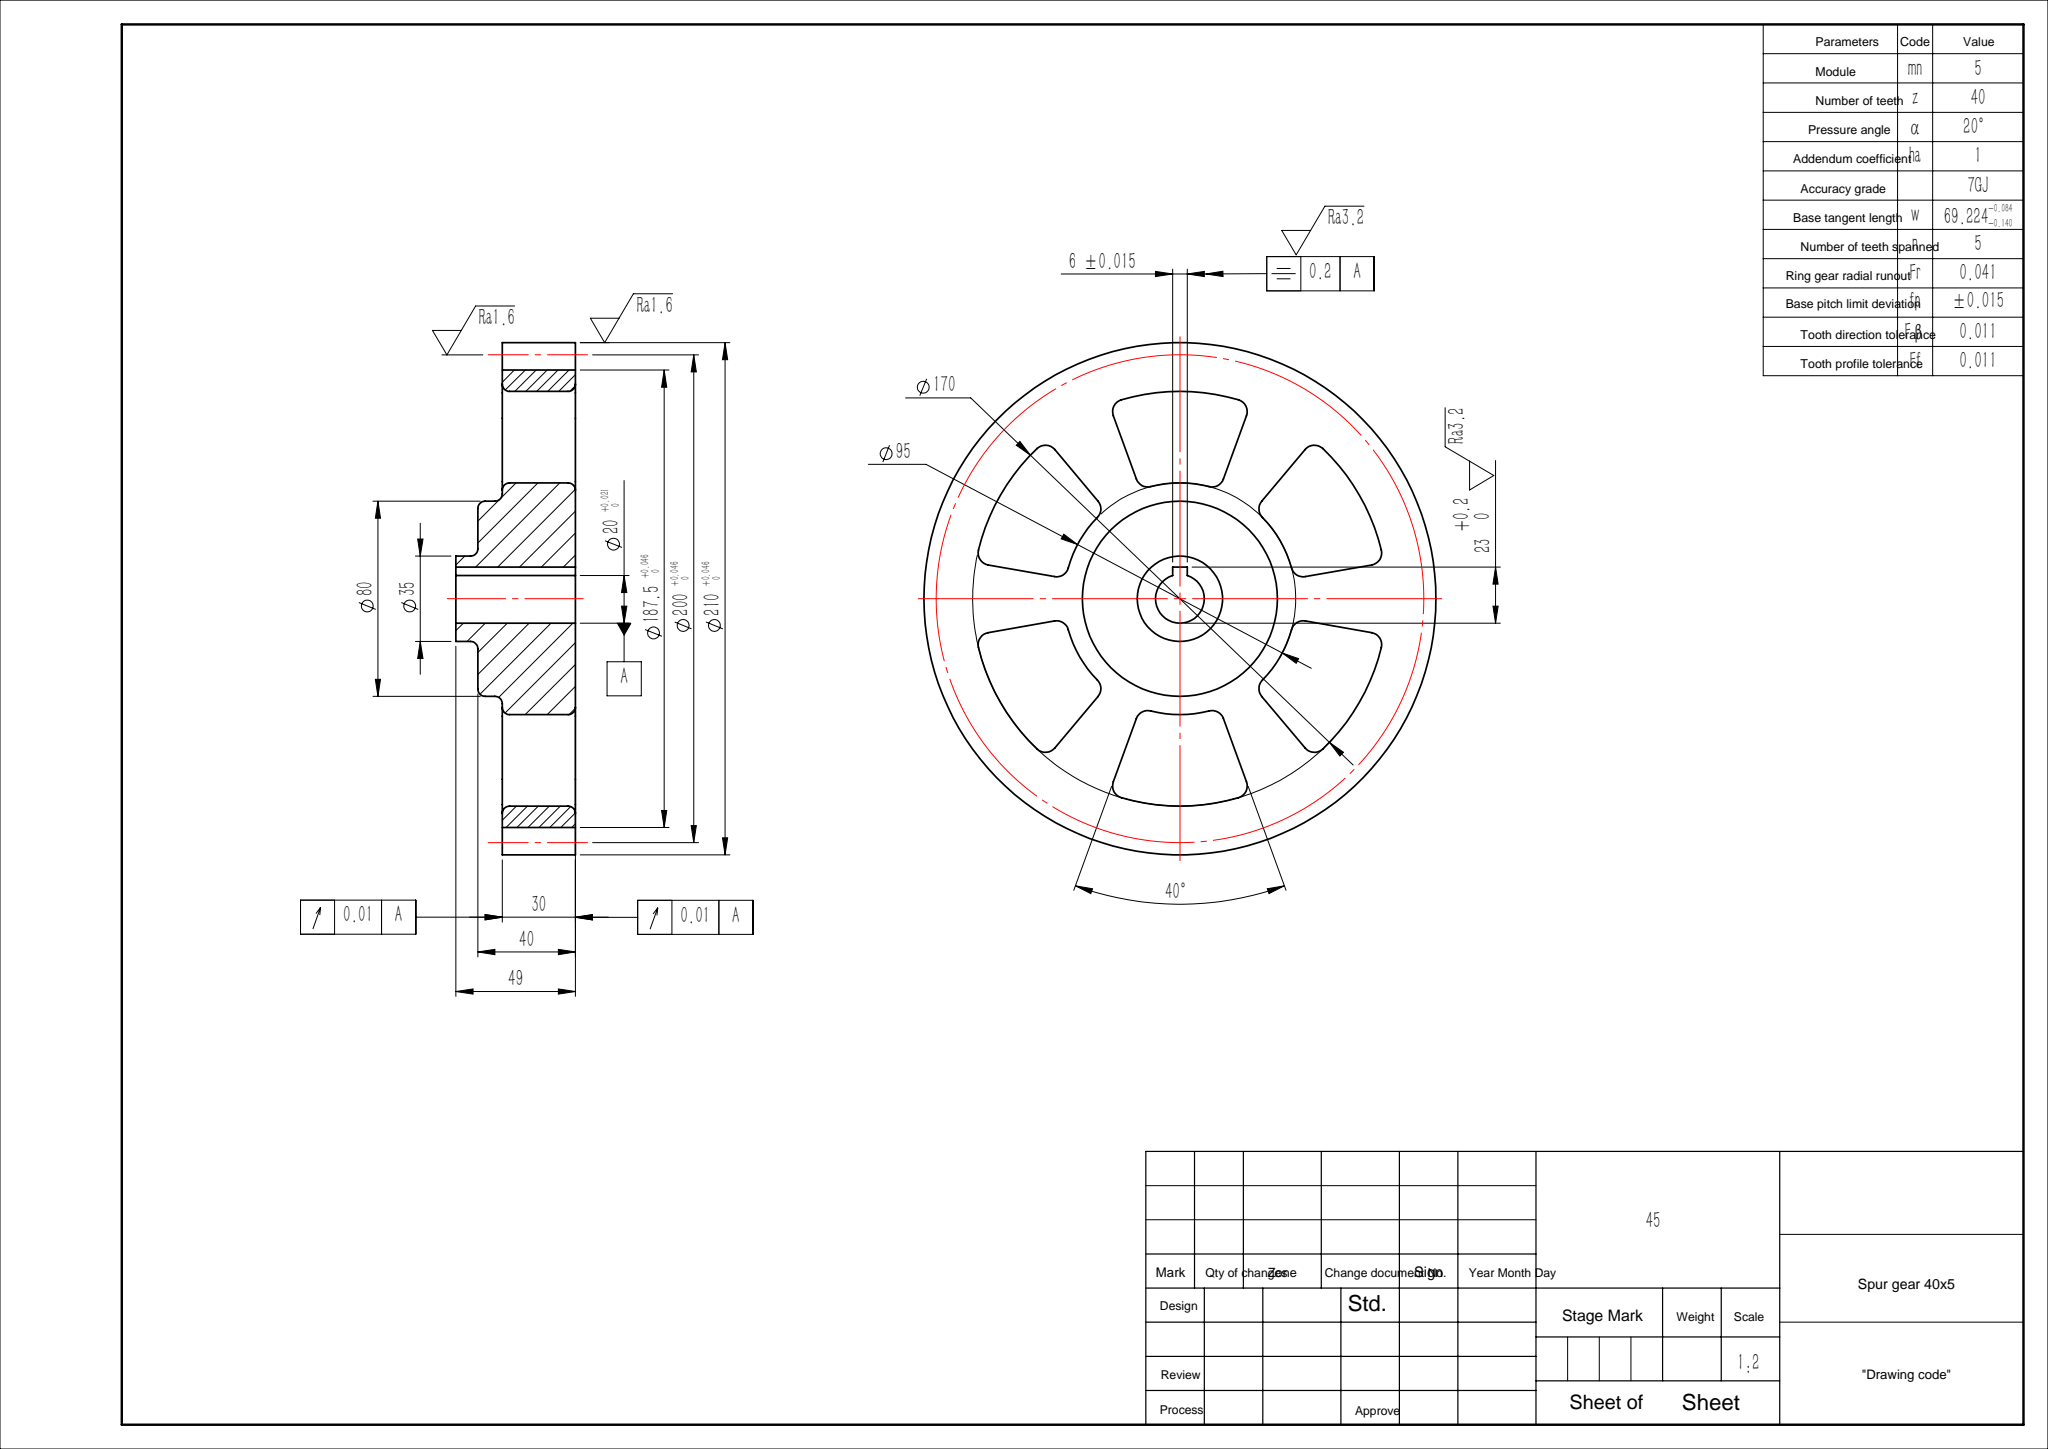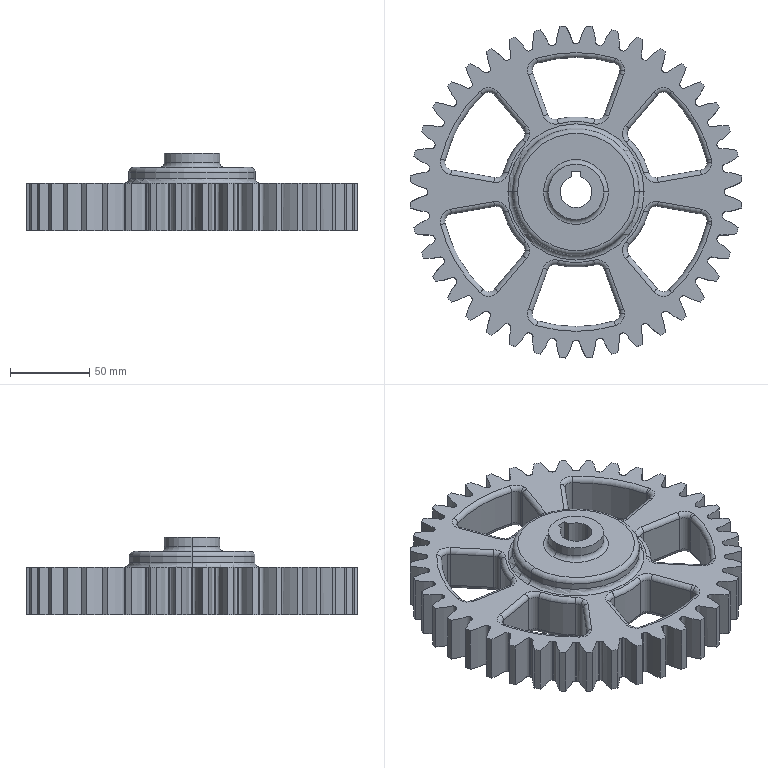Part | SolidWorks | features ICE 5, CirPattern 2, Extrusion 1, Fillet 1, RefAxis 1 | 1 solid | 343 faces | box 209.617 x 209.617 x 49 mm | volume 665029 mm3 | cylinder 154 | torus 90 | spline 80 | plane 19 | commonest cylinder face diameters 187.5 x41 210 x40 10 x30 6 x24 95 x6 170 x6